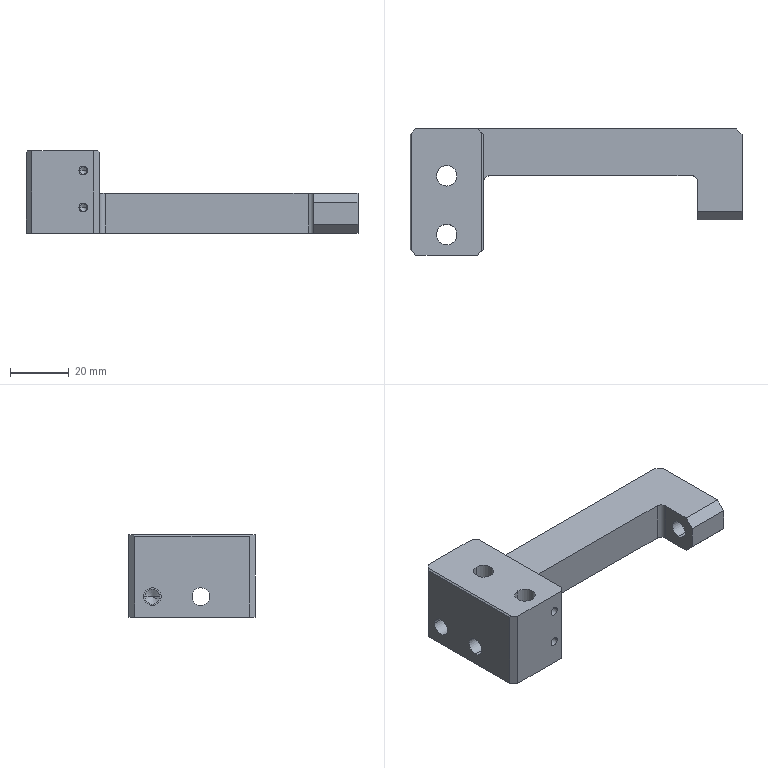Part | STEP file | J454-EBZ05-23-00-Part-1 | 1 solid | 58 faces | box 113 x 43 x 28 mm | volume 47585 mm3 | cylinder 26 | plane 24 | cone 8 | commonest cylinder face diameters 6 x8 2.5 x4 3 x4 5.1 x4 7 x4 4 x2